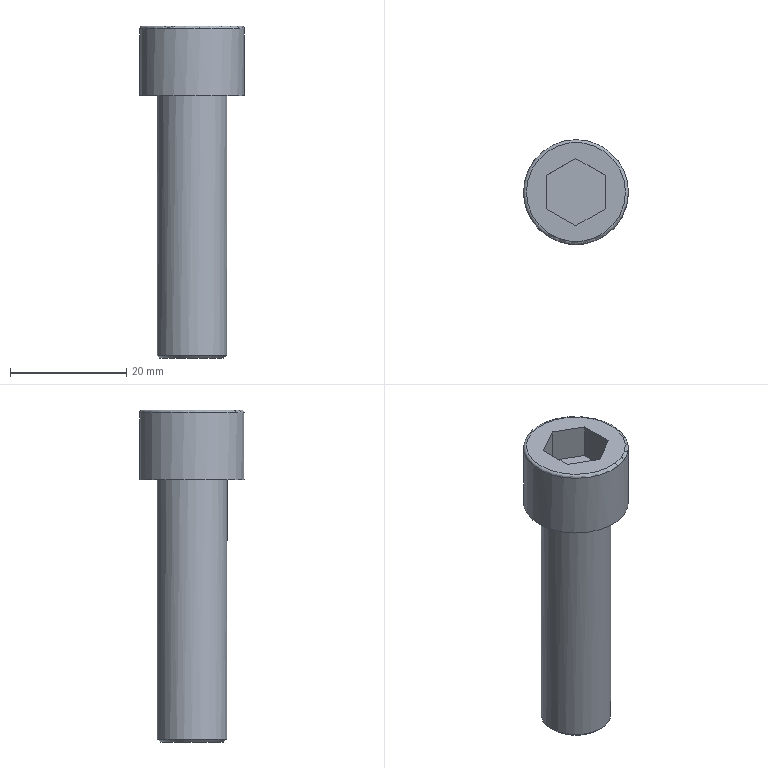Part | NX | features 模具.stp<1>[119] 2 | 1 solid | 14 faces | box 18 x 18 x 57 mm | volume 7616 mm3 | plane 10 | cylinder 2 | cone 1 | torus 1 | commonest cylinder face diameters 12 x1 18 x1
STEP:
#1=CARTESIAN_POINT('',(0.,-214.226,-159.5));
#2=VERTEX_POINT('',#1);
#3=CARTESIAN_POINT('',(-5.,-217.113,-159.5));
#4=VERTEX_POINT('',#3);
#5=CARTESIAN_POINT('',(0.,-214.226,-159.5));
#6=DIRECTION('',(-0.866,-0.5,0.));
#7=VECTOR('',#6,1000.);
#8=LINE('',#5,#7);
#9=EDGE_CURVE('',#2,#4,#8,.T.);
#10=ORIENTED_EDGE('',*,*,#9,.T.);
#11=CARTESIAN_POINT('',(-5.,-222.887,-159.5));
#12=VERTEX_POINT('',#11);
#13=CARTESIAN_POINT('',(-5.,-217.113,-159.5));
#14=DIRECTION('',(0.,-1.,0.));
#15=VECTOR('',#14,1000.);
#16=LINE('',#13,#15);
#17=EDGE_CURVE('',#4,#12,#16,.T.);
#18=ORIENTED_EDGE('',*,*,#17,.T.);
#19=CARTESIAN_POINT('',(0.,-225.774,-159.5));
#20=VERTEX_POINT('',#19);
#21=CARTESIAN_POINT('',(-5.,-222.887,-159.5));
#22=DIRECTION('',(0.866,-0.5,0.));
#23=VECTOR('',#22,1000.);
#24=LINE('',#21,#23);
#25=EDGE_CURVE('',#12,#20,#24,.T.);
#26=ORIENTED_EDGE('',*,*,#25,.T.);
#27=CARTESIAN_POINT('',(5.,-222.887,-159.5));
#28=VERTEX_POINT('',#27);
#29=CARTESIAN_POINT('',(0.,-225.774,-159.5));
#30=DIRECTION('',(0.866,0.5,0.));
#31=VECTOR('',#30,1000.);
#32=LINE('',#29,#31);
#33=EDGE_CURVE('',#20,#28,#32,.T.);
#34=ORIENTED_EDGE('',*,*,#33,.T.);
#35=CARTESIAN_POINT('',(5.,-217.113,-159.5));
#36=VERTEX_POINT('',#35);
#37=CARTESIAN_POINT('',(5.,-222.887,-159.5));
#38=DIRECTION('',(0.,1.,0.));
#39=VECTOR('',#38,1000.);
#40=LINE('',#37,#39);
#41=EDGE_CURVE('',#28,#36,#40,.T.);
#42=ORIENTED_EDGE('',*,*,#41,.T.);
#43=CARTESIAN_POINT('',(5.,-217.113,-159.5));
#44=DIRECTION('',(-0.866,0.5,0.));
#45=VECTOR('',#44,1000.);
#46=LINE('',#43,#45);
#47=EDGE_CURVE('',#36,#2,#46,.T.);
#48=ORIENTED_EDGE('',*,*,#47,.T.);
#49=EDGE_LOOP('',(#10,#18,#26,#34,#42,#48));
#50=FACE_BOUND('',#49,.T.);
#51=CARTESIAN_POINT('',(0.,-220.,-159.5));
#52=DIRECTION('',(0.,0.,-1.));
#53=DIRECTION('',(0.,-1.,0.));
#54=AXIS2_PLACEMENT_3D('',#51,#52,#53);
#55=PLANE('',#54);
#56=ADVANCED_FACE('',(#50),#55,.F.);
#57=CARTESIAN_POINT('',(0.,-214.226,-153.5));
#58=VERTEX_POINT('',#57);
#59=CARTESIAN_POINT('',(-5.,-217.113,-153.5));
#60=VERTEX_POINT('',#59);
#61=CARTESIAN_POINT('',(0.,-214.226,-153.5));
#62=DIRECTION('',(-0.866,-0.5,0.));
#63=VECTOR('',#62,1000.);
#64=LINE('',#61,#63);
#65=EDGE_CURVE('',#58,#60,#64,.T.);
#66=ORIENTED_EDGE('',*,*,#65,.T.);
#67=CARTESIAN_POINT('',(-5.,-217.113,-159.5));
#68=DIRECTION('',(0.,0.,1.));
#69=VECTOR('',#68,1000.);
#70=LINE('',#67,#69);
#71=EDGE_CURVE('',#4,#60,#70,.T.);
#72=ORIENTED_EDGE('',*,*,#71,.F.);
#73=ORIENTED_EDGE('',*,*,#9,.F.);
#74=CARTESIAN_POINT('',(0.,-214.226,-159.5));
#75=DIRECTION('',(0.,0.,1.));
#76=VECTOR('',#75,1000.);
#77=LINE('',#74,#76);
#78=EDGE_CURVE('',#2,#58,#77,.T.);
#79=ORIENTED_EDGE('',*,*,#78,.T.);
#80=EDGE_LOOP('',(#66,#72,#73,#79));
#81=FACE_BOUND('',#80,.T.);
#82=CARTESIAN_POINT('',(-2.5,-215.67,-156.5));
#83=DIRECTION('',(-0.5,0.866,0.));
#84=DIRECTION('',(0.,0.,1.));
#85=AXIS2_PLACEMENT_3D('',#82,#83,#84);
#86=PLANE('',#85);
#87=ADVANCED_FACE('',(#81),#86,.F.);
#88=CARTESIAN_POINT('',(-5.,-222.887,-153.5));
#89=VERTEX_POINT('',#88);
#90=CARTESIAN_POINT('',(-5.,-217.113,-153.5));
#91=DIRECTION('',(0.,-1.,0.));
#92=VECTOR('',#91,1000.);
#93=LINE('',#90,#92);
#94=EDGE_CURVE('',#60,#89,#93,.T.);
#95=ORIENTED_EDGE('',*,*,#94,.T.);
#96=CARTESIAN_POINT('',(-5.,-222.887,-159.5));
#97=DIRECTION('',(0.,0.,1.));
#98=VECTOR('',#97,1000.);
#99=LINE('',#96,#98);
#100=EDGE_CURVE('',#12,#89,#99,.T.);
#101=ORIENTED_EDGE('',*,*,#100,.F.);
#102=ORIENTED_EDGE('',*,*,#17,.F.);
#103=ORIENTED_EDGE('',*,*,#71,.T.);
#104=EDGE_LOOP('',(#95,#101,#102,#103));
#105=FACE_BOUND('',#104,.T.);
#106=CARTESIAN_POINT('',(-5.,-220.,-156.5));
#107=DIRECTION('',(-1.,0.,0.));
#108=DIRECTION('',(0.,1.,0.));
#109=AXIS2_PLACEMENT_3D('',#106,#107,#108);
#110=PLANE('',#109);
#111=ADVANCED_FACE('',(#105),#110,.F.);
#112=CARTESIAN_POINT('',(0.,-225.774,-153.5));
#113=VERTEX_POINT('',#112);
#114=CARTESIAN_POINT('',(-5.,-222.887,-153.5));
#115=DIRECTION('',(0.866,-0.5,0.));
#116=VECTOR('',#115,1000.);
#117=LINE('',#114,#116);
#118=EDGE_CURVE('',#89,#113,#117,.T.);
#119=ORIENTED_EDGE('',*,*,#118,.T.);
#120=CARTESIAN_POINT('',(0.,-225.774,-159.5));
#121=DIRECTION('',(0.,0.,1.));
#122=VECTOR('',#121,1000.);
#123=LINE('',#120,#122);
#124=EDGE_CURVE('',#20,#113,#123,.T.);
#125=ORIENTED_EDGE('',*,*,#124,.F.);
#126=ORIENTED_EDGE('',*,*,#25,.F.);
#127=ORIENTED_EDGE('',*,*,#100,.T.);
#128=EDGE_LOOP('',(#119,#125,#126,#127));
#129=FACE_BOUND('',#128,.T.);
#130=CARTESIAN_POINT('',(-2.5,-224.33,-156.5));
#131=DIRECTION('',(-0.5,-0.866,0.));
#132=DIRECTION('',(-0.866,0.5,0.));
#133=AXIS2_PLACEMENT_3D('',#130,#131,#132);
#134=PLANE('',#133);
#135=ADVANCED_FACE('',(#129),#134,.F.);
#136=CARTESIAN_POINT('',(5.,-222.887,-153.5));
#137=VERTEX_POINT('',#136);
#138=CARTESIAN_POINT('',(0.,-225.774,-153.5));
#139=DIRECTION('',(0.866,0.5,0.));
#140=VECTOR('',#139,1000.);
#141=LINE('',#138,#140);
#142=EDGE_CURVE('',#113,#137,#141,.T.);
#143=ORIENTED_EDGE('',*,*,#142,.T.);
#144=CARTESIAN_POINT('',(5.,-222.887,-159.5));
#145=DIRECTION('',(0.,0.,1.));
#146=VECTOR('',#145,1000.);
#147=LINE('',#144,#146);
#148=EDGE_CURVE('',#28,#137,#147,.T.);
#149=ORIENTED_EDGE('',*,*,#148,.F.);
#150=ORIENTED_EDGE('',*,*,#33,.F.);
#151=ORIENTED_EDGE('',*,*,#124,.T.);
#152=EDGE_LOOP('',(#143,#149,#150,#151));
#153=FACE_BOUND('',#152,.T.);
#154=CARTESIAN_POINT('',(2.5,-224.33,-156.5));
#155=DIRECTION('',(0.5,-0.866,0.));
#156=DIRECTION('',(0.,0.,-1.));
#157=AXIS2_PLACEMENT_3D('',#154,#155,#156);
#158=PLANE('',#157);
#159=ADVANCED_FACE('',(#153),#158,.F.);
#160=CARTESIAN_POINT('',(5.,-217.113,-153.5));
#161=VERTEX_POINT('',#160);
#162=CARTESIAN_POINT('',(5.,-222.887,-153.5));
#163=DIRECTION('',(0.,1.,0.));
#164=VECTOR('',#163,1000.);
#165=LINE('',#162,#164);
#166=EDGE_CURVE('',#137,#161,#165,.T.);
#167=ORIENTED_EDGE('',*,*,#166,.T.);
#168=CARTESIAN_POINT('',(5.,-217.113,-159.5));
#169=DIRECTION('',(0.,0.,1.));
#170=VECTOR('',#169,1000.);
#171=LINE('',#168,#170);
#172=EDGE_CURVE('',#36,#161,#171,.T.);
#173=ORIENTED_EDGE('',*,*,#172,.F.);
#174=ORIENTED_EDGE('',*,*,#41,.F.);
#175=ORIENTED_EDGE('',*,*,#148,.T.);
#176=EDGE_LOOP('',(#167,#173,#174,#175));
#177=FACE_BOUND('',#176,.T.);
#178=CARTESIAN_POINT('',(5.,-220.,-156.5));
#179=DIRECTION('',(1.,0.,0.));
#180=DIRECTION('',(0.,0.,1.));
#181=AXIS2_PLACEMENT_3D('',#178,#179,#180);
#182=PLANE('',#181);
#183=ADVANCED_FACE('',(#177),#182,.F.);
#184=CARTESIAN_POINT('',(5.,-217.113,-153.5));
#185=DIRECTION('',(-0.866,0.5,0.));
#186=VECTOR('',#185,1000.);
#187=LINE('',#184,#186);
#188=EDGE_CURVE('',#161,#58,#187,.T.);
#189=ORIENTED_EDGE('',*,*,#188,.T.);
#190=ORIENTED_EDGE('',*,*,#78,.F.);
#191=ORIENTED_EDGE('',*,*,#47,.F.);
#192=ORIENTED_EDGE('',*,*,#172,.T.);
#193=EDGE_LOOP('',(#189,#190,#191,#192));
#194=FACE_BOUND('',#193,.T.);
#195=CARTESIAN_POINT('',(2.5,-215.67,-156.5));
#196=DIRECTION('',(0.5,0.866,0.));
#197=DIRECTION('',(0.,0.,-1.));
#198=AXIS2_PLACEMENT_3D('',#195,#196,#197);
#199=PLANE('',#198);
#200=ADVANCED_FACE('',(#194),#199,.F.);
#201=CARTESIAN_POINT('',(-6.,-220.,-210.));
#202=VERTEX_POINT('',#201);
#203=CARTESIAN_POINT('',(0.,-220.,-210.));
#204=DIRECTION('',(0.,0.,1.));
#205=DIRECTION('',(-1.,0.,0.));
#206=AXIS2_PLACEMENT_3D('',#203,#204,#205);
#207=CIRCLE('',#206,6.);
#208=EDGE_CURVE('',#202,#202,#207,.T.);
#209=ORIENTED_EDGE('',*,*,#208,.F.);
#210=EDGE_LOOP('',(#209));
#211=FACE_BOUND('',#210,.T.);
#212=CARTESIAN_POINT('',(-5.5,-220.,-210.5));
#213=VERTEX_POINT('',#212);
#214=CARTESIAN_POINT('',(0.,-220.,-210.5));
#215=DIRECTION('',(0.,0.,-1.));
#216=DIRECTION('',(-1.,0.,0.));
#217=AXIS2_PLACEMENT_3D('',#214,#215,#216);
#218=CIRCLE('',#217,5.5);
#219=EDGE_CURVE('',#213,#213,#218,.T.);
#220=ORIENTED_EDGE('',*,*,#219,.F.);
#221=EDGE_LOOP('',(#220));
#222=FACE_BOUND('',#221,.T.);
#223=CARTESIAN_POINT('',(0.,-220.,-210.));
#224=DIRECTION('',(0.,0.,1.));
#225=DIRECTION('',(1.,0.,0.));
#226=AXIS2_PLACEMENT_3D('',#223,#224,#225);
#227=CONICAL_SURFACE('',#226,6.,0.7854);
#228=ADVANCED_FACE('',(#211,#222),#227,.T.);
#229=CARTESIAN_POINT('',(0.,-214.,-165.5));
#230=VERTEX_POINT('',#229);
#231=CARTESIAN_POINT('',(0.,-220.,-165.5));
#232=DIRECTION('',(0.,0.,-1.));
#233=DIRECTION('',(0.,1.,0.));
#234=AXIS2_PLACEMENT_3D('',#231,#232,#233);
#235=CIRCLE('',#234,6.);
#236=EDGE_CURVE('',#230,#230,#235,.T.);
#237=ORIENTED_EDGE('',*,*,#236,.T.);
#238=EDGE_LOOP('',(#237));
#239=FACE_BOUND('',#238,.T.);
#240=ORIENTED_EDGE('',*,*,#208,.T.);
#241=EDGE_LOOP('',(#240));
#242=FACE_BOUND('',#241,.T.);
#243=CARTESIAN_POINT('',(0.,-220.,-205.5));
#244=DIRECTION('',(0.,0.,1.));
#245=DIRECTION('',(0.,1.,0.));
#246=AXIS2_PLACEMENT_3D('',#243,#244,#245);
#247=CYLINDRICAL_SURFACE('',#246,6.);
#248=ADVANCED_FACE('',(#239,#242),#247,.T.);
#249=ORIENTED_EDGE('',*,*,#219,.T.);
#250=EDGE_LOOP('',(#249));
#251=FACE_BOUND('',#250,.T.);
#252=CARTESIAN_POINT('',(0.,-220.,-210.5));
#253=DIRECTION('',(0.,0.,-1.));
#254=DIRECTION('',(0.,-1.,0.));
#255=AXIS2_PLACEMENT_3D('',#252,#253,#254);
#256=PLANE('',#255);
#257=ADVANCED_FACE('',(#251),#256,.T.);
#258=CARTESIAN_POINT('',(9.,-220.,-154.));
#259=VERTEX_POINT('',#258);
#260=CARTESIAN_POINT('',(0.,-220.,-154.));
#261=DIRECTION('',(0.,0.,-1.));
#262=DIRECTION('',(1.,0.,0.));
#263=AXIS2_PLACEMENT_3D('',#260,#261,#262);
#264=CIRCLE('',#263,9.);
#265=EDGE_CURVE('',#259,#259,#264,.T.);
#266=ORIENTED_EDGE('',*,*,#265,.F.);
#267=EDGE_LOOP('',(#266));
#268=FACE_BOUND('',#267,.T.);
#269=CARTESIAN_POINT('',(8.5,-220.,-153.5));
#270=VERTEX_POINT('',#269);
#271=CARTESIAN_POINT('',(0.,-220.,-153.5));
#272=DIRECTION('',(0.,0.,1.));
#273=DIRECTION('',(1.,0.,0.));
#274=AXIS2_PLACEMENT_3D('',#271,#272,#273);
#275=CIRCLE('',#274,8.5);
#276=EDGE_CURVE('',#270,#270,#275,.T.);
#277=ORIENTED_EDGE('',*,*,#276,.F.);
#278=EDGE_LOOP('',(#277));
#279=FACE_BOUND('',#278,.T.);
#280=CARTESIAN_POINT('',(0.,-220.,-154.));
#281=DIRECTION('',(0.,0.,1.));
#282=DIRECTION('',(1.,0.,0.));
#283=AXIS2_PLACEMENT_3D('',#280,#281,#282);
#284=TOROIDAL_SURFACE('',#283,8.5,0.5);
#285=ADVANCED_FACE('',(#268,#279),#284,.T.);
#286=CARTESIAN_POINT('',(0.,-211.,-165.5));
#287=VERTEX_POINT('',#286);
#288=CARTESIAN_POINT('',(0.,-220.,-165.5));
#289=DIRECTION('',(0.,0.,1.));
#290=DIRECTION('',(0.,1.,0.));
#291=AXIS2_PLACEMENT_3D('',#288,#289,#290);
#292=CIRCLE('',#291,9.);
#293=EDGE_CURVE('',#287,#287,#292,.T.);
#294=ORIENTED_EDGE('',*,*,#293,.T.);
#295=EDGE_LOOP('',(#294));
#296=FACE_BOUND('',#295,.T.);
#297=ORIENTED_EDGE('',*,*,#265,.T.);
#298=EDGE_LOOP('',(#297));
#299=FACE_BOUND('',#298,.T.);
#300=CARTESIAN_POINT('',(0.,-220.,-165.5));
#301=DIRECTION('',(0.,0.,1.));
#302=DIRECTION('',(0.,1.,0.));
#303=AXIS2_PLACEMENT_3D('',#300,#301,#302);
#304=CYLINDRICAL_SURFACE('',#303,9.);
#305=ADVANCED_FACE('',(#296,#299),#304,.T.);
#306=ORIENTED_EDGE('',*,*,#293,.F.);
#307=EDGE_LOOP('',(#306));
#308=FACE_BOUND('',#307,.T.);
#309=ORIENTED_EDGE('',*,*,#236,.F.);
#310=EDGE_LOOP('',(#309));
#311=FACE_BOUND('',#310,.T.);
#312=CARTESIAN_POINT('',(0.,-220.,-165.5));
#313=DIRECTION('',(0.,0.,-1.));
#314=DIRECTION('',(0.,-1.,0.));
#315=AXIS2_PLACEMENT_3D('',#312,#313,#314);
#316=PLANE('',#315);
#317=ADVANCED_FACE('',(#308,#311),#316,.T.);
#318=ORIENTED_EDGE('',*,*,#276,.T.);
#319=EDGE_LOOP('',(#318));
#320=FACE_BOUND('',#319,.T.);
#321=ORIENTED_EDGE('',*,*,#188,.F.);
#322=ORIENTED_EDGE('',*,*,#166,.F.);
#323=ORIENTED_EDGE('',*,*,#142,.F.);
#324=ORIENTED_EDGE('',*,*,#118,.F.);
#325=ORIENTED_EDGE('',*,*,#94,.F.);
#326=ORIENTED_EDGE('',*,*,#65,.F.);
#327=EDGE_LOOP('',(#321,#322,#323,#324,#325,#326));
#328=FACE_BOUND('',#327,.T.);
#329=CARTESIAN_POINT('',(0.,-220.,-153.5));
#330=DIRECTION('',(0.,0.,1.));
#331=DIRECTION('',(1.,0.,0.));
#332=AXIS2_PLACEMENT_3D('',#329,#330,#331);
#333=PLANE('',#332);
#334=ADVANCED_FACE('',(#320,#328),#333,.T.);
#335=CLOSED_SHELL('',(#56,#87,#111,#135,#159,#183,#200,#228,#248,#257,#285,#305,#317,#334));
#336=MANIFOLD_SOLID_BREP('',#335);
#337=(LENGTH_UNIT()NAMED_UNIT(*)SI_UNIT(.MILLI.,.METRE.));
#338=UNCERTAINTY_MEASURE_WITH_UNIT(LENGTH_MEASURE(0.00001),#337,'','');
#339=(NAMED_UNIT(*)PLANE_ANGLE_UNIT()SI_UNIT($,.RADIAN.));
#340=(NAMED_UNIT(*)SI_UNIT($,.STERADIAN.)SOLID_ANGLE_UNIT());
#341=(GEOMETRIC_REPRESENTATION_CONTEXT(3)GLOBAL_UNCERTAINTY_ASSIGNED_CONTEXT((#338))GLOBAL_UNIT_ASSIGNED_CONTEXT((#337,#339,#340))REPRESENTATION_CONTEXT('',''));
#342=ADVANCED_BREP_SHAPE_REPRESENTATION('',(#336),#341);